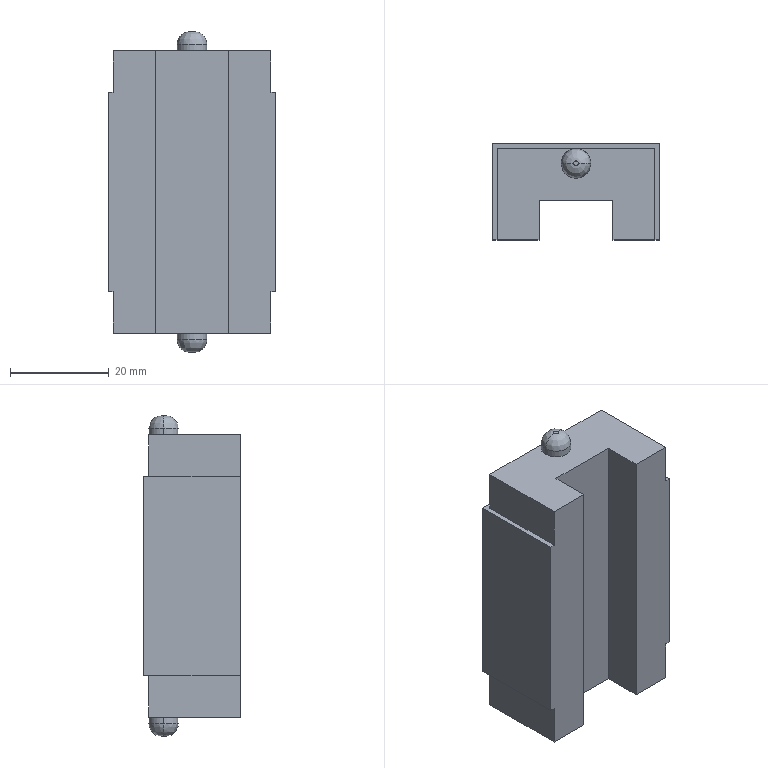Part | STEP file | 1 solid | 44 faces | box 34 x 19.5 x 65 mm | volume 29765 mm3 | plane 20 | cylinder 12 | cone 8 | other 4 | commonest cylinder face diameters 3.3 x8 6 x4